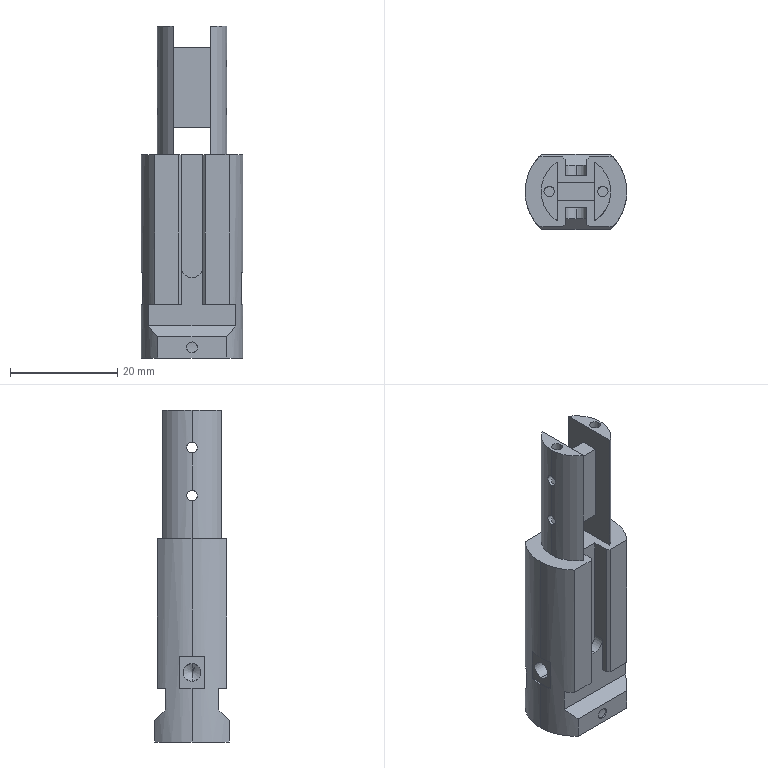Part | STEP file | magnetizing head 2-2 | 1 solid | 94 faces | box 19 x 14 x 62 mm | volume 8649 mm3 | cylinder 48 | plane 42 | cone 4 | commonest cylinder face diameters 2 x32 3.3 x4 4 x4 13 x3 19 x3 13.57 x2